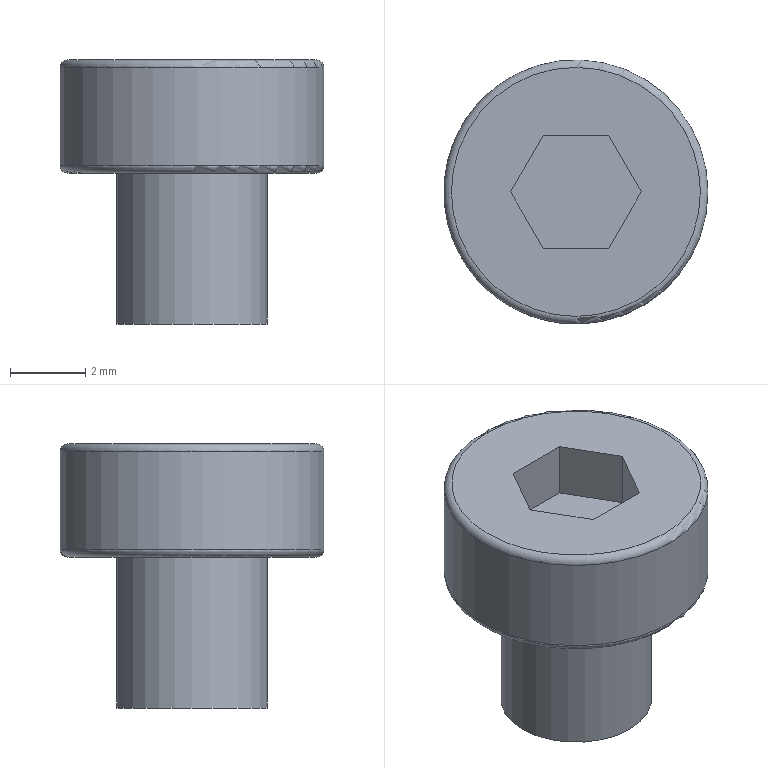Part | STEP file | Tube feed_id802_x_t | 1 solid | 14 faces | box 7 x 7 x 7 mm | volume 153.655 mm3 | plane 10 | cylinder 2 | torus 2 | commonest cylinder face diameters 4 x1 7 x1
STEP:
#1=CARTESIAN_POINT('',(0.,0.,0.));
#2=DIRECTION('',(0.,0.,1.));
#3=DIRECTION('',(1.,0.,0.));
#4=AXIS2_PLACEMENT_3D('',#1,#2,#3);
#5=CARTESIAN_POINT('',(457.,3.036,-9.8));
#6=VERTEX_POINT('',#5);
#7=CARTESIAN_POINT('',(453.5,3.036,-9.8));
#8=DIRECTION('',(0.,0.,1.));
#9=DIRECTION('',(1.,0.,0.));
#10=AXIS2_PLACEMENT_3D('',#7,#8,#9);
#11=CIRCLE('',#10,3.5);
#12=CARTESIAN_POINT('',(453.5,3.036,-10.));
#13=DIRECTION('',(0.,0.,1.));
#14=DIRECTION('',(1.,0.,0.));
#15=AXIS2_PLACEMENT_3D('',#12,#13,#14);
#16=CYLINDRICAL_SURFACE('',#15,3.5);
#17=CARTESIAN_POINT('',(0.,0.2));
#18=DIRECTION('',(1.,0.));
#19=VECTOR('',#18,1.);
#20=LINE('',#17,#19);
#21=(GEOMETRIC_REPRESENTATION_CONTEXT(2)PARAMETRIC_REPRESENTATION_CONTEXT()REPRESENTATION_CONTEXT('',''));
#22=DEFINITIONAL_REPRESENTATION('',(#20),#21);
#23=PCURVE('',#16,#22);
#24=CARTESIAN_POINT('',(453.5,3.036,-9.8));
#25=DIRECTION('',(0.,0.,1.));
#26=DIRECTION('',(1.,0.,0.));
#27=AXIS2_PLACEMENT_3D('',#24,#25,#26);
#28=TOROIDAL_SURFACE('',#27,3.3,0.2);
#29=CARTESIAN_POINT('',(0.,6.283));
#30=DIRECTION('',(1.,0.));
#31=VECTOR('',#30,1.);
#32=LINE('',#29,#31);
#33=(GEOMETRIC_REPRESENTATION_CONTEXT(2)PARAMETRIC_REPRESENTATION_CONTEXT()REPRESENTATION_CONTEXT('',''));
#34=DEFINITIONAL_REPRESENTATION('',(#32),#33);
#35=PCURVE('',#28,#34);
#36=SURFACE_CURVE('',#11,(#23,#35),.PCURVE_S1.);
#37=EDGE_CURVE('',#6,#6,#36,.T.);
#38=ORIENTED_EDGE('',*,*,#37,.T.);
#39=CARTESIAN_POINT('',(457.,3.036,-7.2));
#40=VERTEX_POINT('',#39);
#41=CARTESIAN_POINT('',(457.,3.036,-9.8));
#42=CARTESIAN_POINT('',(457.,3.036,-7.2));
#43=B_SPLINE_CURVE_WITH_KNOTS('',1,(#41,#42),.UNSPECIFIED.,.F.,.F.,(2,2),(0.2,2.8),.PIECEWISE_BEZIER_KNOTS.);
#44=CARTESIAN_POINT('',(6.283,0.));
#45=DIRECTION('',(0.,1.));
#46=VECTOR('',#45,1.);
#47=LINE('',#44,#46);
#48=(GEOMETRIC_REPRESENTATION_CONTEXT(2)PARAMETRIC_REPRESENTATION_CONTEXT()REPRESENTATION_CONTEXT('',''));
#49=DEFINITIONAL_REPRESENTATION('',(#47),#48);
#50=PCURVE('',#16,#49);
#51=CARTESIAN_POINT('',(0.,0.));
#52=DIRECTION('',(0.,1.));
#53=VECTOR('',#52,1.);
#54=LINE('',#51,#53);
#55=(GEOMETRIC_REPRESENTATION_CONTEXT(2)PARAMETRIC_REPRESENTATION_CONTEXT()REPRESENTATION_CONTEXT('',''));
#56=DEFINITIONAL_REPRESENTATION('',(#54),#55);
#57=PCURVE('',#16,#56);
#58=SEAM_CURVE('',#43,(#50,#57),.PCURVE_S1.);
#59=EDGE_CURVE('',#6,#40,#58,.T.);
#60=ORIENTED_EDGE('',*,*,#59,.T.);
#61=CARTESIAN_POINT('',(453.5,3.036,-7.2));
#62=DIRECTION('',(0.,0.,-1.));
#63=DIRECTION('',(1.,0.,0.));
#64=AXIS2_PLACEMENT_3D('',#61,#62,#63);
#65=CIRCLE('',#64,3.5);
#66=CARTESIAN_POINT('',(6.283,2.8));
#67=DIRECTION('',(-1.,0.));
#68=VECTOR('',#67,1.);
#69=LINE('',#66,#68);
#70=(GEOMETRIC_REPRESENTATION_CONTEXT(2)PARAMETRIC_REPRESENTATION_CONTEXT()REPRESENTATION_CONTEXT('',''));
#71=DEFINITIONAL_REPRESENTATION('',(#69),#70);
#72=PCURVE('',#16,#71);
#73=CARTESIAN_POINT('',(453.5,3.036,-7.2));
#74=DIRECTION('',(0.,0.,1.));
#75=DIRECTION('',(1.,0.,0.));
#76=AXIS2_PLACEMENT_3D('',#73,#74,#75);
#77=TOROIDAL_SURFACE('',#76,3.3,0.2);
#78=CARTESIAN_POINT('',(6.283,6.283));
#79=DIRECTION('',(-1.,0.));
#80=VECTOR('',#79,1.);
#81=LINE('',#78,#80);
#82=(GEOMETRIC_REPRESENTATION_CONTEXT(2)PARAMETRIC_REPRESENTATION_CONTEXT()REPRESENTATION_CONTEXT('',''));
#83=DEFINITIONAL_REPRESENTATION('',(#81),#82);
#84=PCURVE('',#77,#83);
#85=SURFACE_CURVE('',#65,(#72,#84),.PCURVE_S1.);
#86=EDGE_CURVE('',#40,#40,#85,.T.);
#87=ORIENTED_EDGE('',*,*,#86,.T.);
#88=ORIENTED_EDGE('',*,*,#59,.F.);
#89=EDGE_LOOP('',(#38,#60,#87,#88));
#90=FACE_BOUND('',#89,.T.);
#91=ADVANCED_FACE('',(#90),#16,.T.);
#92=CARTESIAN_POINT('',(451.5,3.036,-10.));
#93=VERTEX_POINT('',#92);
#94=CARTESIAN_POINT('',(453.5,3.036,-10.));
#95=DIRECTION('',(0.,0.,-1.));
#96=DIRECTION('',(-1.,0.,0.));
#97=AXIS2_PLACEMENT_3D('',#94,#95,#96);
#98=CIRCLE('',#97,2.);
#99=CARTESIAN_POINT('',(453.5,3.036,-10.));
#100=DIRECTION('',(0.,0.,1.));
#101=DIRECTION('',(1.,0.,0.));
#102=AXIS2_PLACEMENT_3D('',#99,#100,#101);
#103=PLANE('',#102);
#104=CARTESIAN_POINT('',(-2.,0.));
#105=CARTESIAN_POINT('',(-2.,3.464));
#106=CARTESIAN_POINT('',(1.,1.732));
#107=CARTESIAN_POINT('',(4.,0.));
#108=CARTESIAN_POINT('',(1.,-1.732));
#109=CARTESIAN_POINT('',(-2.,-3.464));
#110=CARTESIAN_POINT('',(-2.,0.));
#111=(BOUNDED_CURVE()B_SPLINE_CURVE(2,(#104,#105,#106,#107,#108,#109,#110),.UNSPECIFIED.,.T.,.F.)B_SPLINE_CURVE_WITH_KNOTS((1,2,2,2,2,1),(-2.094,0.,2.094,4.189,6.283,8.378),.UNSPECIFIED.)CURVE()GEOMETRIC_REPRESENTATION_ITEM()RATIONAL_B_SPLINE_CURVE((1.,0.5,1.,0.5,1.,0.5,1.))REPRESENTATION_ITEM(''));
#112=(GEOMETRIC_REPRESENTATION_CONTEXT(2)PARAMETRIC_REPRESENTATION_CONTEXT()REPRESENTATION_CONTEXT('',''));
#113=DEFINITIONAL_REPRESENTATION('',(#111),#112);
#114=PCURVE('',#103,#113);
#115=CARTESIAN_POINT('',(453.5,3.036,-14.));
#116=DIRECTION('',(0.,0.,1.));
#117=DIRECTION('',(1.,0.,0.));
#118=AXIS2_PLACEMENT_3D('',#115,#116,#117);
#119=CYLINDRICAL_SURFACE('',#118,2.);
#120=CARTESIAN_POINT('',(9.425,4.));
#121=DIRECTION('',(-1.,0.));
#122=VECTOR('',#121,1.);
#123=LINE('',#120,#122);
#124=(GEOMETRIC_REPRESENTATION_CONTEXT(2)PARAMETRIC_REPRESENTATION_CONTEXT()REPRESENTATION_CONTEXT('',''));
#125=DEFINITIONAL_REPRESENTATION('',(#123),#124);
#126=PCURVE('',#119,#125);
#127=SURFACE_CURVE('',#98,(#114,#126),.PCURVE_S1.);
#128=EDGE_CURVE('',#93,#93,#127,.T.);
#129=ORIENTED_EDGE('',*,*,#128,.F.);
#130=EDGE_LOOP('',(#129));
#131=FACE_BOUND('',#130,.T.);
#132=CARTESIAN_POINT('',(456.8,3.036,-10.));
#133=VERTEX_POINT('',#132);
#134=CARTESIAN_POINT('',(453.5,3.036,-10.));
#135=DIRECTION('',(0.,0.,-1.));
#136=DIRECTION('',(1.,0.,0.));
#137=AXIS2_PLACEMENT_3D('',#134,#135,#136);
#138=CIRCLE('',#137,3.3);
#139=CARTESIAN_POINT('',(3.3,0.));
#140=CARTESIAN_POINT('',(3.3,-5.716));
#141=CARTESIAN_POINT('',(-1.65,-2.858));
#142=CARTESIAN_POINT('',(-6.6,0.));
#143=CARTESIAN_POINT('',(-1.65,2.858));
#144=CARTESIAN_POINT('',(3.3,5.716));
#145=CARTESIAN_POINT('',(3.3,0.));
#146=(BOUNDED_CURVE()B_SPLINE_CURVE(2,(#139,#140,#141,#142,#143,#144,#145),.UNSPECIFIED.,.T.,.F.)B_SPLINE_CURVE_WITH_KNOTS((1,2,2,2,2,1),(-2.094,0.,2.094,4.189,6.283,8.378),.UNSPECIFIED.)CURVE()GEOMETRIC_REPRESENTATION_ITEM()RATIONAL_B_SPLINE_CURVE((1.,0.5,1.,0.5,1.,0.5,1.))REPRESENTATION_ITEM(''));
#147=(GEOMETRIC_REPRESENTATION_CONTEXT(2)PARAMETRIC_REPRESENTATION_CONTEXT()REPRESENTATION_CONTEXT('',''));
#148=DEFINITIONAL_REPRESENTATION('',(#146),#147);
#149=PCURVE('',#103,#148);
#150=CARTESIAN_POINT('',(6.283,4.712));
#151=DIRECTION('',(-1.,0.));
#152=VECTOR('',#151,1.);
#153=LINE('',#150,#152);
#154=(GEOMETRIC_REPRESENTATION_CONTEXT(2)PARAMETRIC_REPRESENTATION_CONTEXT()REPRESENTATION_CONTEXT('',''));
#155=DEFINITIONAL_REPRESENTATION('',(#153),#154);
#156=PCURVE('',#28,#155);
#157=SURFACE_CURVE('',#138,(#149,#156),.PCURVE_S1.);
#158=EDGE_CURVE('',#133,#133,#157,.T.);
#159=ORIENTED_EDGE('',*,*,#158,.T.);
#160=EDGE_LOOP('',(#159));
#161=FACE_BOUND('',#160,.T.);
#162=ADVANCED_FACE('',(#131,#161),#103,.F.);
#163=CARTESIAN_POINT('',(451.768,3.036,-7.));
#164=VERTEX_POINT('',#163);
#165=CARTESIAN_POINT('',(452.634,1.536,-7.));
#166=VERTEX_POINT('',#165);
#167=CARTESIAN_POINT('',(451.768,3.036,-7.));
#168=DIRECTION('',(0.5,-0.866,0.));
#169=VECTOR('',#168,1.);
#170=LINE('',#167,#169);
#171=CARTESIAN_POINT('',(453.5,3.036,-7.));
#172=DIRECTION('',(0.,0.,1.));
#173=DIRECTION('',(1.,0.,0.));
#174=AXIS2_PLACEMENT_3D('',#171,#172,#173);
#175=PLANE('',#174);
#176=CARTESIAN_POINT('',(-1.732,0.));
#177=DIRECTION('',(0.5,-0.866));
#178=VECTOR('',#177,1.);
#179=LINE('',#176,#178);
#180=(GEOMETRIC_REPRESENTATION_CONTEXT(2)PARAMETRIC_REPRESENTATION_CONTEXT()REPRESENTATION_CONTEXT('',''));
#181=DEFINITIONAL_REPRESENTATION('',(#179),#180);
#182=PCURVE('',#175,#181);
#183=CARTESIAN_POINT('',(451.768,3.036,-8.5));
#184=DIRECTION('',(-0.866,-0.5,0.));
#185=DIRECTION('',(0.5,-0.866,0.));
#186=AXIS2_PLACEMENT_3D('',#183,#184,#185);
#187=PLANE('',#186);
#188=CARTESIAN_POINT('',(0.,1.5));
#189=DIRECTION('',(1.,0.));
#190=VECTOR('',#189,1.);
#191=LINE('',#188,#190);
#192=(GEOMETRIC_REPRESENTATION_CONTEXT(2)PARAMETRIC_REPRESENTATION_CONTEXT()REPRESENTATION_CONTEXT('',''));
#193=DEFINITIONAL_REPRESENTATION('',(#191),#192);
#194=PCURVE('',#187,#193);
#195=SURFACE_CURVE('',#170,(#182,#194),.PCURVE_S1.);
#196=EDGE_CURVE('',#164,#166,#195,.T.);
#197=ORIENTED_EDGE('',*,*,#196,.F.);
#198=CARTESIAN_POINT('',(452.634,4.536,-7.));
#199=VERTEX_POINT('',#198);
#200=CARTESIAN_POINT('',(452.634,4.536,-7.));
#201=DIRECTION('',(-0.5,-0.866,0.));
#202=VECTOR('',#201,1.);
#203=LINE('',#200,#202);
#204=CARTESIAN_POINT('',(-0.866,1.5));
#205=DIRECTION('',(-0.5,-0.866));
#206=VECTOR('',#205,1.);
#207=LINE('',#204,#206);
#208=(GEOMETRIC_REPRESENTATION_CONTEXT(2)PARAMETRIC_REPRESENTATION_CONTEXT()REPRESENTATION_CONTEXT('',''));
#209=DEFINITIONAL_REPRESENTATION('',(#207),#208);
#210=PCURVE('',#175,#209);
#211=CARTESIAN_POINT('',(452.634,4.536,-8.5));
#212=DIRECTION('',(-0.866,0.5,0.));
#213=DIRECTION('',(-0.5,-0.866,0.));
#214=AXIS2_PLACEMENT_3D('',#211,#212,#213);
#215=PLANE('',#214);
#216=CARTESIAN_POINT('',(0.,1.5));
#217=DIRECTION('',(1.,0.));
#218=VECTOR('',#217,1.);
#219=LINE('',#216,#218);
#220=(GEOMETRIC_REPRESENTATION_CONTEXT(2)PARAMETRIC_REPRESENTATION_CONTEXT()REPRESENTATION_CONTEXT('',''));
#221=DEFINITIONAL_REPRESENTATION('',(#219),#220);
#222=PCURVE('',#215,#221);
#223=SURFACE_CURVE('',#203,(#210,#222),.PCURVE_S1.);
#224=EDGE_CURVE('',#199,#164,#223,.T.);
#225=ORIENTED_EDGE('',*,*,#224,.F.);
#226=CARTESIAN_POINT('',(454.366,4.536,-7.));
#227=VERTEX_POINT('',#226);
#228=CARTESIAN_POINT('',(454.366,4.536,-7.));
#229=DIRECTION('',(-1.,0.,0.));
#230=VECTOR('',#229,1.);
#231=LINE('',#228,#230);
#232=CARTESIAN_POINT('',(0.866,1.5));
#233=DIRECTION('',(-1.,0.));
#234=VECTOR('',#233,1.);
#235=LINE('',#232,#234);
#236=(GEOMETRIC_REPRESENTATION_CONTEXT(2)PARAMETRIC_REPRESENTATION_CONTEXT()REPRESENTATION_CONTEXT('',''));
#237=DEFINITIONAL_REPRESENTATION('',(#235),#236);
#238=PCURVE('',#175,#237);
#239=CARTESIAN_POINT('',(454.366,4.536,-8.5));
#240=DIRECTION('',(0.,1.,0.));
#241=DIRECTION('',(0.,0.,1.));
#242=AXIS2_PLACEMENT_3D('',#239,#240,#241);
#243=PLANE('',#242);
#244=CARTESIAN_POINT('',(1.5,0.));
#245=DIRECTION('',(0.,-1.));
#246=VECTOR('',#245,1.);
#247=LINE('',#244,#246);
#248=(GEOMETRIC_REPRESENTATION_CONTEXT(2)PARAMETRIC_REPRESENTATION_CONTEXT()REPRESENTATION_CONTEXT('',''));
#249=DEFINITIONAL_REPRESENTATION('',(#247),#248);
#250=PCURVE('',#243,#249);
#251=SURFACE_CURVE('',#231,(#238,#250),.PCURVE_S1.);
#252=EDGE_CURVE('',#227,#199,#251,.T.);
#253=ORIENTED_EDGE('',*,*,#252,.F.);
#254=CARTESIAN_POINT('',(455.232,3.036,-7.));
#255=VERTEX_POINT('',#254);
#256=CARTESIAN_POINT('',(455.232,3.036,-7.));
#257=DIRECTION('',(-0.5,0.866,0.));
#258=VECTOR('',#257,1.);
#259=LINE('',#256,#258);
#260=CARTESIAN_POINT('',(1.732,0.));
#261=DIRECTION('',(-0.5,0.866));
#262=VECTOR('',#261,1.);
#263=LINE('',#260,#262);
#264=(GEOMETRIC_REPRESENTATION_CONTEXT(2)PARAMETRIC_REPRESENTATION_CONTEXT()REPRESENTATION_CONTEXT('',''));
#265=DEFINITIONAL_REPRESENTATION('',(#263),#264);
#266=PCURVE('',#175,#265);
#267=CARTESIAN_POINT('',(455.232,3.036,-8.5));
#268=DIRECTION('',(0.866,0.5,0.));
#269=DIRECTION('',(-0.5,0.866,0.));
#270=AXIS2_PLACEMENT_3D('',#267,#268,#269);
#271=PLANE('',#270);
#272=CARTESIAN_POINT('',(0.,1.5));
#273=DIRECTION('',(1.,0.));
#274=VECTOR('',#273,1.);
#275=LINE('',#272,#274);
#276=(GEOMETRIC_REPRESENTATION_CONTEXT(2)PARAMETRIC_REPRESENTATION_CONTEXT()REPRESENTATION_CONTEXT('',''));
#277=DEFINITIONAL_REPRESENTATION('',(#275),#276);
#278=PCURVE('',#271,#277);
#279=SURFACE_CURVE('',#259,(#266,#278),.PCURVE_S1.);
#280=EDGE_CURVE('',#255,#227,#279,.T.);
#281=ORIENTED_EDGE('',*,*,#280,.F.);
#282=CARTESIAN_POINT('',(454.366,1.536,-7.));
#283=VERTEX_POINT('',#282);
#284=CARTESIAN_POINT('',(454.366,1.536,-7.));
#285=DIRECTION('',(0.5,0.866,0.));
#286=VECTOR('',#285,1.);
#287=LINE('',#284,#286);
#288=CARTESIAN_POINT('',(0.866,-1.5));
#289=DIRECTION('',(0.5,0.866));
#290=VECTOR('',#289,1.);
#291=LINE('',#288,#290);
#292=(GEOMETRIC_REPRESENTATION_CONTEXT(2)PARAMETRIC_REPRESENTATION_CONTEXT()REPRESENTATION_CONTEXT('',''));
#293=DEFINITIONAL_REPRESENTATION('',(#291),#292);
#294=PCURVE('',#175,#293);
#295=CARTESIAN_POINT('',(454.366,1.536,-8.5));
#296=DIRECTION('',(0.866,-0.5,0.));
#297=DIRECTION('',(0.5,0.866,0.));
#298=AXIS2_PLACEMENT_3D('',#295,#296,#297);
#299=PLANE('',#298);
#300=CARTESIAN_POINT('',(0.,1.5));
#301=DIRECTION('',(1.,0.));
#302=VECTOR('',#301,1.);
#303=LINE('',#300,#302);
#304=(GEOMETRIC_REPRESENTATION_CONTEXT(2)PARAMETRIC_REPRESENTATION_CONTEXT()REPRESENTATION_CONTEXT('',''));
#305=DEFINITIONAL_REPRESENTATION('',(#303),#304);
#306=PCURVE('',#299,#305);
#307=SURFACE_CURVE('',#287,(#294,#306),.PCURVE_S1.);
#308=EDGE_CURVE('',#283,#255,#307,.T.);
#309=ORIENTED_EDGE('',*,*,#308,.F.);
#310=CARTESIAN_POINT('',(452.634,1.536,-7.));
#311=DIRECTION('',(1.,0.,0.));
#312=VECTOR('',#311,1.);
#313=LINE('',#310,#312);
#314=CARTESIAN_POINT('',(-0.866,-1.5));
#315=DIRECTION('',(1.,0.));
#316=VECTOR('',#315,1.);
#317=LINE('',#314,#316);
#318=(GEOMETRIC_REPRESENTATION_CONTEXT(2)PARAMETRIC_REPRESENTATION_CONTEXT()REPRESENTATION_CONTEXT('',''));
#319=DEFINITIONAL_REPRESENTATION('',(#317),#318);
#320=PCURVE('',#175,#319);
#321=CARTESIAN_POINT('',(452.634,1.536,-8.5));
#322=DIRECTION('',(0.,-1.,0.));
#323=DIRECTION('',(0.,0.,-1.));
#324=AXIS2_PLACEMENT_3D('',#321,#322,#323);
#325=PLANE('',#324);
#326=CARTESIAN_POINT('',(-1.5,0.));
#327=DIRECTION('',(0.,1.));
#328=VECTOR('',#327,1.);
#329=LINE('',#326,#328);
#330=(GEOMETRIC_REPRESENTATION_CONTEXT(2)PARAMETRIC_REPRESENTATION_CONTEXT()REPRESENTATION_CONTEXT('',''));
#331=DEFINITIONAL_REPRESENTATION('',(#329),#330);
#332=PCURVE('',#325,#331);
#333=SURFACE_CURVE('',#313,(#320,#332),.PCURVE_S1.);
#334=EDGE_CURVE('',#166,#283,#333,.T.);
#335=ORIENTED_EDGE('',*,*,#334,.F.);
#336=EDGE_LOOP('',(#197,#225,#253,#281,#309,#335));
#337=FACE_BOUND('',#336,.T.);
#338=CARTESIAN_POINT('',(456.8,3.036,-7.));
#339=VERTEX_POINT('',#338);
#340=CARTESIAN_POINT('',(453.5,3.036,-7.));
#341=DIRECTION('',(0.,0.,1.));
#342=DIRECTION('',(1.,0.,0.));
#343=AXIS2_PLACEMENT_3D('',#340,#341,#342);
#344=CIRCLE('',#343,3.3);
#345=CARTESIAN_POINT('',(0.,0.));
#346=DIRECTION('',(1.,0.));
#347=AXIS2_PLACEMENT_2D('',#345,#346);
#348=CIRCLE('',#347,3.3);
#349=(GEOMETRIC_REPRESENTATION_CONTEXT(2)PARAMETRIC_REPRESENTATION_CONTEXT()REPRESENTATION_CONTEXT('',''));
#350=DEFINITIONAL_REPRESENTATION('',(#348),#349);
#351=PCURVE('',#175,#350);
#352=CARTESIAN_POINT('',(0.,7.854));
#353=DIRECTION('',(1.,0.));
#354=VECTOR('',#353,1.);
#355=LINE('',#352,#354);
#356=(GEOMETRIC_REPRESENTATION_CONTEXT(2)PARAMETRIC_REPRESENTATION_CONTEXT()REPRESENTATION_CONTEXT('',''));
#357=DEFINITIONAL_REPRESENTATION('',(#355),#356);
#358=PCURVE('',#77,#357);
#359=SURFACE_CURVE('',#344,(#351,#358),.PCURVE_S1.);
#360=EDGE_CURVE('',#339,#339,#359,.T.);
#361=ORIENTED_EDGE('',*,*,#360,.T.);
#362=EDGE_LOOP('',(#361));
#363=FACE_BOUND('',#362,.T.);
#364=ADVANCED_FACE('',(#337,#363),#175,.T.);
#365=ORIENTED_EDGE('',*,*,#158,.F.);
#366=CARTESIAN_POINT('',(456.8,3.036,-10.));
#367=CARTESIAN_POINT('',(456.853,3.036,-10.));
#368=CARTESIAN_POINT('',(456.906,3.036,-9.983));
#369=CARTESIAN_POINT('',(456.95,3.036,-9.95));
#370=CARTESIAN_POINT('',(456.983,3.036,-9.906));
#371=CARTESIAN_POINT('',(457.,3.036,-9.853));
#372=CARTESIAN_POINT('',(457.,3.036,-9.8));
#373=(BOUNDED_CURVE()B_SPLINE_CURVE(6,(#366,#367,#368,#369,#370,#371,#372),.UNSPECIFIED.,.F.,.F.)B_SPLINE_CURVE_WITH_KNOTS((7,7),(4.712,6.283),.PIECEWISE_BEZIER_KNOTS.)CURVE()GEOMETRIC_REPRESENTATION_ITEM()RATIONAL_B_SPLINE_CURVE((1.031,1.01,0.9979,0.994,0.9979,1.01,1.031))REPRESENTATION_ITEM(''));
#374=CARTESIAN_POINT('',(6.283,0.));
#375=DIRECTION('',(0.,1.));
#376=VECTOR('',#375,1.);
#377=LINE('',#374,#376);
#378=(GEOMETRIC_REPRESENTATION_CONTEXT(2)PARAMETRIC_REPRESENTATION_CONTEXT()REPRESENTATION_CONTEXT('',''));
#379=DEFINITIONAL_REPRESENTATION('',(#377),#378);
#380=PCURVE('',#28,#379);
#381=CARTESIAN_POINT('',(0.,0.));
#382=DIRECTION('',(0.,1.));
#383=VECTOR('',#382,1.);
#384=LINE('',#381,#383);
#385=(GEOMETRIC_REPRESENTATION_CONTEXT(2)PARAMETRIC_REPRESENTATION_CONTEXT()REPRESENTATION_CONTEXT('',''));
#386=DEFINITIONAL_REPRESENTATION('',(#384),#385);
#387=PCURVE('',#28,#386);
#388=SEAM_CURVE('',#373,(#380,#387),.PCURVE_S1.);
#389=EDGE_CURVE('',#133,#6,#388,.T.);
#390=ORIENTED_EDGE('',*,*,#389,.T.);
#391=ORIENTED_EDGE('',*,*,#37,.F.);
#392=ORIENTED_EDGE('',*,*,#389,.F.);
#393=EDGE_LOOP('',(#365,#390,#391,#392));
#394=FACE_BOUND('',#393,.T.);
#395=ADVANCED_FACE('',(#394),#28,.T.);
#396=ORIENTED_EDGE('',*,*,#86,.F.);
#397=CARTESIAN_POINT('',(457.,3.036,-7.2));
#398=CARTESIAN_POINT('',(457.,3.036,-7.147));
#399=CARTESIAN_POINT('',(456.983,3.036,-7.094));
#400=CARTESIAN_POINT('',(456.95,3.036,-7.05));
#401=CARTESIAN_POINT('',(456.906,3.036,-7.017));
#402=CARTESIAN_POINT('',(456.853,3.036,-7.));
#403=CARTESIAN_POINT('',(456.8,3.036,-7.));
#404=(BOUNDED_CURVE()B_SPLINE_CURVE(6,(#397,#398,#399,#400,#401,#402,#403),.UNSPECIFIED.,.F.,.F.)B_SPLINE_CURVE_WITH_KNOTS((7,7),(0.,1.571),.PIECEWISE_BEZIER_KNOTS.)CURVE()GEOMETRIC_REPRESENTATION_ITEM()RATIONAL_B_SPLINE_CURVE((1.031,1.01,0.9979,0.994,0.9979,1.01,1.031))REPRESENTATION_ITEM(''));
#405=CARTESIAN_POINT('',(6.283,6.283));
#406=DIRECTION('',(0.,1.));
#407=VECTOR('',#406,1.);
#408=LINE('',#405,#407);
#409=(GEOMETRIC_REPRESENTATION_CONTEXT(2)PARAMETRIC_REPRESENTATION_CONTEXT()REPRESENTATION_CONTEXT('',''));
#410=DEFINITIONAL_REPRESENTATION('',(#408),#409);
#411=PCURVE('',#77,#410);
#412=CARTESIAN_POINT('',(0.,6.283));
#413=DIRECTION('',(0.,1.));
#414=VECTOR('',#413,1.);
#415=LINE('',#412,#414);
#416=(GEOMETRIC_REPRESENTATION_CONTEXT(2)PARAMETRIC_REPRESENTATION_CONTEXT()REPRESENTATION_CONTEXT('',''));
#417=DEFINITIONAL_REPRESENTATION('',(#415),#416);
#418=PCURVE('',#77,#417);
#419=SEAM_CURVE('',#404,(#411,#418),.PCURVE_S1.);
#420=EDGE_CURVE('',#40,#339,#419,.T.);
#421=ORIENTED_EDGE('',*,*,#420,.T.);
#422=ORIENTED_EDGE('',*,*,#360,.F.);
#423=ORIENTED_EDGE('',*,*,#420,.F.);
#424=EDGE_LOOP('',(#396,#421,#422,#423));
#425=FACE_BOUND('',#424,.T.);
#426=ADVANCED_FACE('',(#425),#77,.T.);
#427=ORIENTED_EDGE('',*,*,#196,.T.);
#428=CARTESIAN_POINT('',(452.634,1.536,-8.5));
#429=VERTEX_POINT('',#428);
#430=CARTESIAN_POINT('',(452.634,1.536,-8.5));
#431=DIRECTION('',(0.,0.,-1.));
#432=VECTOR('',#431,1.);
#433=LINE('',#430,#432);
#434=CARTESIAN_POINT('',(1.732,0.));
#435=DIRECTION('',(0.,-1.));
#436=VECTOR('',#435,1.);
#437=LINE('',#434,#436);
#438=(GEOMETRIC_REPRESENTATION_CONTEXT(2)PARAMETRIC_REPRESENTATION_CONTEXT()REPRESENTATION_CONTEXT('',''));
#439=DEFINITIONAL_REPRESENTATION('',(#437),#438);
#440=PCURVE('',#187,#439);
#441=CARTESIAN_POINT('',(0.,0.));
#442=DIRECTION('',(1.,0.));
#443=VECTOR('',#442,1.);
#444=LINE('',#441,#443);
#445=(GEOMETRIC_REPRESENTATION_CONTEXT(2)PARAMETRIC_REPRESENTATION_CONTEXT()REPRESENTATION_CONTEXT('',''));
#446=DEFINITIONAL_REPRESENTATION('',(#444),#445);
#447=PCURVE('',#325,#446);
#448=SURFACE_CURVE('',#433,(#440,#447),.PCURVE_S1.);
#449=EDGE_CURVE('',#166,#429,#448,.T.);
#450=ORIENTED_EDGE('',*,*,#449,.T.);
#451=CARTESIAN_POINT('',(451.768,3.036,-8.5));
#452=VERTEX_POINT('',#451);
#453=CARTESIAN_POINT('',(451.768,3.036,-8.5));
#454=DIRECTION('',(-0.5,0.866,0.));
#455=VECTOR('',#454,1.);
#456=LINE('',#453,#455);
#457=CARTESIAN_POINT('',(0.,0.));
#458=DIRECTION('',(-1.,0.));
#459=VECTOR('',#458,1.);
#460=LINE('',#457,#459);
#461=(GEOMETRIC_REPRESENTATION_CONTEXT(2)PARAMETRIC_REPRESENTATION_CONTEXT()REPRESENTATION_CONTEXT('',''));
#462=DEFINITIONAL_REPRESENTATION('',(#460),#461);
#463=PCURVE('',#187,#462);
#464=CARTESIAN_POINT('',(0.,0.,-8.5));
#465=DIRECTION('',(0.,0.,1.));
#466=DIRECTION('',(1.,0.,0.));
#467=AXIS2_PLACEMENT_3D('',#464,#465,#466);
#468=PLANE('',#467);
#469=CARTESIAN_POINT('',(451.768,3.036));
#470=DIRECTION('',(-0.5,0.866));
#471=VECTOR('',#470,1.);
#472=LINE('',#469,#471);
#473=(GEOMETRIC_REPRESENTATION_CONTEXT(2)PARAMETRIC_REPRESENTATION_CONTEXT()REPRESENTATION_CONTEXT('',''));
#474=DEFINITIONAL_REPRESENTATION('',(#472),#473);
#475=PCURVE('',#468,#474);
#476=SURFACE_CURVE('',#456,(#463,#475),.PCURVE_S1.);
#477=EDGE_CURVE('',#429,#452,#476,.T.);
#478=ORIENTED_EDGE('',*,*,#477,.T.);
#479=CARTESIAN_POINT('',(451.768,3.036,-8.5));
#480=DIRECTION('',(0.,0.,-1.));
#481=VECTOR('',#480,1.);
#482=LINE('',#479,#481);
#483=CARTESIAN_POINT('',(0.,0.));
#484=DIRECTION('',(0.,-1.));
#485=VECTOR('',#484,1.);
#486=LINE('',#483,#485);
#487=(GEOMETRIC_REPRESENTATION_CONTEXT(2)PARAMETRIC_REPRESENTATION_CONTEXT()REPRESENTATION_CONTEXT('',''));
#488=DEFINITIONAL_REPRESENTATION('',(#486),#487);
#489=PCURVE('',#187,#488);
#490=CARTESIAN_POINT('',(1.732,0.));
#491=DIRECTION('',(0.,-1.));
#492=VECTOR('',#491,1.);
#493=LINE('',#490,#492);
#494=(GEOMETRIC_REPRESENTATION_CONTEXT(2)PARAMETRIC_REPRESENTATION_CONTEXT()REPRESENTATION_CONTEXT('',''));
#495=DEFINITIONAL_REPRESENTATION('',(#493),#494);
#496=PCURVE('',#215,#495);
#497=SURFACE_CURVE('',#482,(#489,#496),.PCURVE_S1.);
#498=EDGE_CURVE('',#164,#452,#497,.T.);
#499=ORIENTED_EDGE('',*,*,#498,.F.);
#500=EDGE_LOOP('',(#427,#450,#478,#499));
#501=FACE_BOUND('',#500,.T.);
#502=ADVANCED_FACE('',(#501),#187,.F.);
#503=ORIENTED_EDGE('',*,*,#334,.T.);
#504=CARTESIAN_POINT('',(454.366,1.536,-8.5));
#505=VERTEX_POINT('',#504);
#506=CARTESIAN_POINT('',(454.366,1.536,-8.5));
#507=DIRECTION('',(0.,0.,-1.));
#508=VECTOR('',#507,1.);
#509=LINE('',#506,#508);
#510=CARTESIAN_POINT('',(0.,1.732));
#511=DIRECTION('',(1.,0.));
#512=VECTOR('',#511,1.);
#513=LINE('',#510,#512);
#514=(GEOMETRIC_REPRESENTATION_CONTEXT(2)PARAMETRIC_REPRESENTATION_CONTEXT()REPRESENTATION_CONTEXT('',''));
#515=DEFINITIONAL_REPRESENTATION('',(#513),#514);
#516=PCURVE('',#325,#515);
#517=CARTESIAN_POINT('',(0.,0.));
#518=DIRECTION('',(0.,-1.));
#519=VECTOR('',#518,1.);
#520=LINE('',#517,#519);
#521=(GEOMETRIC_REPRESENTATION_CONTEXT(2)PARAMETRIC_REPRESENTATION_CONTEXT()REPRESENTATION_CONTEXT('',''));
#522=DEFINITIONAL_REPRESENTATION('',(#520),#521);
#523=PCURVE('',#299,#522);
#524=SURFACE_CURVE('',#509,(#516,#523),.PCURVE_S1.);
#525=EDGE_CURVE('',#283,#505,#524,.T.);
#526=ORIENTED_EDGE('',*,*,#525,.T.);
#527=CARTESIAN_POINT('',(452.634,1.536,-8.5));
#528=DIRECTION('',(-1.,0.,0.));
#529=VECTOR('',#528,1.);
#530=LINE('',#527,#529);
#531=CARTESIAN_POINT('',(0.,0.));
#532=DIRECTION('',(0.,-1.));
#533=VECTOR('',#532,1.);
#534=LINE('',#531,#533);
#535=(GEOMETRIC_REPRESENTATION_CONTEXT(2)PARAMETRIC_REPRESENTATION_CONTEXT()REPRESENTATION_CONTEXT('',''));
#536=DEFINITIONAL_REPRESENTATION('',(#534),#535);
#537=PCURVE('',#325,#536);
#538=CARTESIAN_POINT('',(452.634,1.536));
#539=DIRECTION('',(-1.,0.));
#540=VECTOR('',#539,1.);
#541=LINE('',#538,#540);
#542=(GEOMETRIC_REPRESENTATION_CONTEXT(2)PARAMETRIC_REPRESENTATION_CONTEXT()REPRESENTATION_CONTEXT('',''));
#543=DEFINITIONAL_REPRESENTATION('',(#541),#542);
#544=PCURVE('',#468,#543);
#545=SURFACE_CURVE('',#530,(#537,#544),.PCURVE_S1.);
#546=EDGE_CURVE('',#505,#429,#545,.T.);
#547=ORIENTED_EDGE('',*,*,#546,.T.);
#548=ORIENTED_EDGE('',*,*,#449,.F.);
#549=EDGE_LOOP('',(#503,#526,#547,#548));
#550=FACE_BOUND('',#549,.T.);
#551=ADVANCED_FACE('',(#550),#325,.F.);
#552=ORIENTED_EDGE('',*,*,#308,.T.);
#553=CARTESIAN_POINT('',(455.232,3.036,-8.5));
#554=VERTEX_POINT('',#553);
#555=CARTESIAN_POINT('',(455.232,3.036,-8.5));
#556=DIRECTION('',(0.,0.,-1.));
#557=VECTOR('',#556,1.);
#558=LINE('',#555,#557);
#559=CARTESIAN_POINT('',(1.732,0.));
#560=DIRECTION('',(0.,-1.));
#561=VECTOR('',#560,1.);
#562=LINE('',#559,#561);
#563=(GEOMETRIC_REPRESENTATION_CONTEXT(2)PARAMETRIC_REPRESENTATION_CONTEXT()REPRESENTATION_CONTEXT('',''));
#564=DEFINITIONAL_REPRESENTATION('',(#562),#563);
#565=PCURVE('',#299,#564);
#566=CARTESIAN_POINT('',(0.,0.));
#567=DIRECTION('',(0.,-1.));
#568=VECTOR('',#567,1.);
#569=LINE('',#566,#568);
#570=(GEOMETRIC_REPRESENTATION_CONTEXT(2)PARAMETRIC_REPRESENTATION_CONTEXT()REPRESENTATION_CONTEXT('',''));
#571=DEFINITIONAL_REPRESENTATION('',(#569),#570);
#572=PCURVE('',#271,#571);
#573=SURFACE_CURVE('',#558,(#565,#572),.PCURVE_S1.);
#574=EDGE_CURVE('',#255,#554,#573,.T.);
#575=ORIENTED_EDGE('',*,*,#574,.T.);
#576=CARTESIAN_POINT('',(454.366,1.536,-8.5));
#577=DIRECTION('',(-0.5,-0.866,0.));
#578=VECTOR('',#577,1.);
#579=LINE('',#576,#578);
#580=CARTESIAN_POINT('',(0.,0.));
#581=DIRECTION('',(-1.,0.));
#582=VECTOR('',#581,1.);
#583=LINE('',#580,#582);
#584=(GEOMETRIC_REPRESENTATION_CONTEXT(2)PARAMETRIC_REPRESENTATION_CONTEXT()REPRESENTATION_CONTEXT('',''));
#585=DEFINITIONAL_REPRESENTATION('',(#583),#584);
#586=PCURVE('',#299,#585);
#587=CARTESIAN_POINT('',(454.366,1.536));
#588=DIRECTION('',(-0.5,-0.866));
#589=VECTOR('',#588,1.);
#590=LINE('',#587,#589);
#591=(GEOMETRIC_REPRESENTATION_CONTEXT(2)PARAMETRIC_REPRESENTATION_CONTEXT()REPRESENTATION_CONTEXT('',''));
#592=DEFINITIONAL_REPRESENTATION('',(#590),#591);
#593=PCURVE('',#468,#592);
#594=SURFACE_CURVE('',#579,(#586,#593),.PCURVE_S1.);
#595=EDGE_CURVE('',#554,#505,#594,.T.);
#596=ORIENTED_EDGE('',*,*,#595,.T.);
#597=ORIENTED_EDGE('',*,*,#525,.F.);
#598=EDGE_LOOP('',(#552,#575,#596,#597));
#599=FACE_BOUND('',#598,.T.);
#600=ADVANCED_FACE('',(#599),#299,.F.);
#601=ORIENTED_EDGE('',*,*,#280,.T.);
#602=CARTESIAN_POINT('',(454.366,4.536,-8.5));
#603=VERTEX_POINT('',#602);
#604=CARTESIAN_POINT('',(454.366,4.536,-8.5));
#605=DIRECTION('',(0.,0.,-1.));
#606=VECTOR('',#605,1.);
#607=LINE('',#604,#606);
#608=CARTESIAN_POINT('',(1.732,0.));
#609=DIRECTION('',(0.,-1.));
#610=VECTOR('',#609,1.);
#611=LINE('',#608,#610);
#612=(GEOMETRIC_REPRESENTATION_CONTEXT(2)PARAMETRIC_REPRESENTATION_CONTEXT()REPRESENTATION_CONTEXT('',''));
#613=DEFINITIONAL_REPRESENTATION('',(#611),#612);
#614=PCURVE('',#271,#613);
#615=CARTESIAN_POINT('',(0.,0.));
#616=DIRECTION('',(-1.,0.));
#617=VECTOR('',#616,1.);
#618=LINE('',#615,#617);
#619=(GEOMETRIC_REPRESENTATION_CONTEXT(2)PARAMETRIC_REPRESENTATION_CONTEXT()REPRESENTATION_CONTEXT('',''));
#620=DEFINITIONAL_REPRESENTATION('',(#618),#619);
#621=PCURVE('',#243,#620);
#622=SURFACE_CURVE('',#607,(#614,#621),.PCURVE_S1.);
#623=EDGE_CURVE('',#227,#603,#622,.T.);
#624=ORIENTED_EDGE('',*,*,#623,.T.);
#625=CARTESIAN_POINT('',(455.232,3.036,-8.5));
#626=DIRECTION('',(0.5,-0.866,0.));
#627=VECTOR('',#626,1.);
#628=LINE('',#625,#627);
#629=CARTESIAN_POINT('',(0.,0.));
#630=DIRECTION('',(-1.,0.));
#631=VECTOR('',#630,1.);
#632=LINE('',#629,#631);
#633=(GEOMETRIC_REPRESENTATION_CONTEXT(2)PARAMETRIC_REPRESENTATION_CONTEXT()REPRESENTATION_CONTEXT('',''));
#634=DEFINITIONAL_REPRESENTATION('',(#632),#633);
#635=PCURVE('',#271,#634);
#636=CARTESIAN_POINT('',(455.232,3.036));
#637=DIRECTION('',(0.5,-0.866));
#638=VECTOR('',#637,1.);
#639=LINE('',#636,#638);
#640=(GEOMETRIC_REPRESENTATION_CONTEXT(2)PARAMETRIC_REPRESENTATION_CONTEXT()REPRESENTATION_CONTEXT('',''));
#641=DEFINITIONAL_REPRESENTATION('',(#639),#640);
#642=PCURVE('',#468,#641);
#643=SURFACE_CURVE('',#628,(#635,#642),.PCURVE_S1.);
#644=EDGE_CURVE('',#603,#554,#643,.T.);
#645=ORIENTED_EDGE('',*,*,#644,.T.);
#646=ORIENTED_EDGE('',*,*,#574,.F.);
#647=EDGE_LOOP('',(#601,#624,#645,#646));
#648=FACE_BOUND('',#647,.T.);
#649=ADVANCED_FACE('',(#648),#271,.F.);
#650=ORIENTED_EDGE('',*,*,#252,.T.);
#651=CARTESIAN_POINT('',(452.634,4.536,-8.5));
#652=VERTEX_POINT('',#651);
#653=CARTESIAN_POINT('',(452.634,4.536,-8.5));
#654=DIRECTION('',(0.,0.,-1.));
#655=VECTOR('',#654,1.);
#656=LINE('',#653,#655);
#657=CARTESIAN_POINT('',(0.,-1.732));
#658=DIRECTION('',(-1.,0.));
#659=VECTOR('',#658,1.);
#660=LINE('',#657,#659);
#661=(GEOMETRIC_REPRESENTATION_CONTEXT(2)PARAMETRIC_REPRESENTATION_CONTEXT()REPRESENTATION_CONTEXT('',''));
#662=DEFINITIONAL_REPRESENTATION('',(#660),#661);
#663=PCURVE('',#243,#662);
#664=CARTESIAN_POINT('',(0.,0.));
#665=DIRECTION('',(0.,-1.));
#666=VECTOR('',#665,1.);
#667=LINE('',#664,#666);
#668=(GEOMETRIC_REPRESENTATION_CONTEXT(2)PARAMETRIC_REPRESENTATION_CONTEXT()REPRESENTATION_CONTEXT('',''));
#669=DEFINITIONAL_REPRESENTATION('',(#667),#668);
#670=PCURVE('',#215,#669);
#671=SURFACE_CURVE('',#656,(#663,#670),.PCURVE_S1.);
#672=EDGE_CURVE('',#199,#652,#671,.T.);
#673=ORIENTED_EDGE('',*,*,#672,.T.);
#674=CARTESIAN_POINT('',(454.366,4.536,-8.5));
#675=DIRECTION('',(1.,0.,0.));
#676=VECTOR('',#675,1.);
#677=LINE('',#674,#676);
#678=CARTESIAN_POINT('',(0.,0.));
#679=DIRECTION('',(0.,1.));
#680=VECTOR('',#679,1.);
#681=LINE('',#678,#680);
#682=(GEOMETRIC_REPRESENTATION_CONTEXT(2)PARAMETRIC_REPRESENTATION_CONTEXT()REPRESENTATION_CONTEXT('',''));
#683=DEFINITIONAL_REPRESENTATION('',(#681),#682);
#684=PCURVE('',#243,#683);
#685=CARTESIAN_POINT('',(454.366,4.536));
#686=DIRECTION('',(1.,0.));
#687=VECTOR('',#686,1.);
#688=LINE('',#685,#687);
#689=(GEOMETRIC_REPRESENTATION_CONTEXT(2)PARAMETRIC_REPRESENTATION_CONTEXT()REPRESENTATION_CONTEXT('',''));
#690=DEFINITIONAL_REPRESENTATION('',(#688),#689);
#691=PCURVE('',#468,#690);
#692=SURFACE_CURVE('',#677,(#684,#691),.PCURVE_S1.);
#693=EDGE_CURVE('',#652,#603,#692,.T.);
#694=ORIENTED_EDGE('',*,*,#693,.T.);
#695=ORIENTED_EDGE('',*,*,#623,.F.);
#696=EDGE_LOOP('',(#650,#673,#694,#695));
#697=FACE_BOUND('',#696,.T.);
#698=ADVANCED_FACE('',(#697),#243,.F.);
#699=ORIENTED_EDGE('',*,*,#224,.T.);
#700=ORIENTED_EDGE('',*,*,#498,.T.);
#701=CARTESIAN_POINT('',(452.634,4.536,-8.5));
#702=DIRECTION('',(0.5,0.866,0.));
#703=VECTOR('',#702,1.);
#704=LINE('',#701,#703);
#705=CARTESIAN_POINT('',(0.,0.));
#706=DIRECTION('',(-1.,0.));
#707=VECTOR('',#706,1.);
#708=LINE('',#705,#707);
#709=(GEOMETRIC_REPRESENTATION_CONTEXT(2)PARAMETRIC_REPRESENTATION_CONTEXT()REPRESENTATION_CONTEXT('',''));
#710=DEFINITIONAL_REPRESENTATION('',(#708),#709);
#711=PCURVE('',#215,#710);
#712=CARTESIAN_POINT('',(452.634,4.536));
#713=DIRECTION('',(0.5,0.866));
#714=VECTOR('',#713,1.);
#715=LINE('',#712,#714);
#716=(GEOMETRIC_REPRESENTATION_CONTEXT(2)PARAMETRIC_REPRESENTATION_CONTEXT()REPRESENTATION_CONTEXT('',''));
#717=DEFINITIONAL_REPRESENTATION('',(#715),#716);
#718=PCURVE('',#468,#717);
#719=SURFACE_CURVE('',#704,(#711,#718),.PCURVE_S1.);
#720=EDGE_CURVE('',#452,#652,#719,.T.);
#721=ORIENTED_EDGE('',*,*,#720,.T.);
#722=ORIENTED_EDGE('',*,*,#672,.F.);
#723=EDGE_LOOP('',(#699,#700,#721,#722));
#724=FACE_BOUND('',#723,.T.);
#725=ADVANCED_FACE('',(#724),#215,.F.);
#726=ORIENTED_EDGE('',*,*,#477,.F.);
#727=ORIENTED_EDGE('',*,*,#546,.F.);
#728=ORIENTED_EDGE('',*,*,#595,.F.);
#729=ORIENTED_EDGE('',*,*,#644,.F.);
#730=ORIENTED_EDGE('',*,*,#693,.F.);
#731=ORIENTED_EDGE('',*,*,#720,.F.);
#732=EDGE_LOOP('',(#726,#727,#728,#729,#730,#731));
#733=FACE_BOUND('',#732,.T.);
#734=ADVANCED_FACE('',(#733),#468,.T.);
#735=CARTESIAN_POINT('',(451.5,3.036,-14.));
#736=VERTEX_POINT('',#735);
#737=CARTESIAN_POINT('',(453.5,3.036,-14.));
#738=DIRECTION('',(0.,0.,-1.));
#739=DIRECTION('',(-1.,0.,0.));
#740=AXIS2_PLACEMENT_3D('',#737,#738,#739);
#741=CIRCLE('',#740,2.);
#742=CARTESIAN_POINT('',(9.425,0.));
#743=DIRECTION('',(-1.,0.));
#744=VECTOR('',#743,1.);
#745=LINE('',#742,#744);
#746=(GEOMETRIC_REPRESENTATION_CONTEXT(2)PARAMETRIC_REPRESENTATION_CONTEXT()REPRESENTATION_CONTEXT('',''));
#747=DEFINITIONAL_REPRESENTATION('',(#745),#746);
#748=PCURVE('',#119,#747);
#749=CARTESIAN_POINT('',(453.5,3.036,-14.));
#750=DIRECTION('',(0.,0.,-1.));
#751=DIRECTION('',(-1.,0.,0.));
#752=AXIS2_PLACEMENT_3D('',#749,#750,#751);
#753=PLANE('',#752);
#754=CARTESIAN_POINT('',(0.,0.));
#755=DIRECTION('',(1.,0.));
#756=AXIS2_PLACEMENT_2D('',#754,#755);
#757=CIRCLE('',#756,2.);
#758=(GEOMETRIC_REPRESENTATION_CONTEXT(2)PARAMETRIC_REPRESENTATION_CONTEXT()REPRESENTATION_CONTEXT('',''));
#759=DEFINITIONAL_REPRESENTATION('',(#757),#758);
#760=PCURVE('',#753,#759);
#761=SURFACE_CURVE('',#741,(#748,#760),.PCURVE_S1.);
#762=EDGE_CURVE('',#736,#736,#761,.T.);
#763=ORIENTED_EDGE('',*,*,#762,.F.);
#764=CARTESIAN_POINT('',(451.5,3.036,-14.));
#765=CARTESIAN_POINT('',(451.5,3.036,-10.));
#766=B_SPLINE_CURVE_WITH_KNOTS('',1,(#764,#765),.UNSPECIFIED.,.F.,.F.,(2,2),(0.,4.),.PIECEWISE_BEZIER_KNOTS.);
#767=CARTESIAN_POINT('',(9.425,0.));
#768=DIRECTION('',(0.,1.));
#769=VECTOR('',#768,1.);
#770=LINE('',#767,#769);
#771=(GEOMETRIC_REPRESENTATION_CONTEXT(2)PARAMETRIC_REPRESENTATION_CONTEXT()REPRESENTATION_CONTEXT('',''));
#772=DEFINITIONAL_REPRESENTATION('',(#770),#771);
#773=PCURVE('',#119,#772);
#774=CARTESIAN_POINT('',(3.142,0.));
#775=DIRECTION('',(0.,1.));
#776=VECTOR('',#775,1.);
#777=LINE('',#774,#776);
#778=(GEOMETRIC_REPRESENTATION_CONTEXT(2)PARAMETRIC_REPRESENTATION_CONTEXT()REPRESENTATION_CONTEXT('',''));
#779=DEFINITIONAL_REPRESENTATION('',(#777),#778);
#780=PCURVE('',#119,#779);
#781=SEAM_CURVE('',#766,(#773,#780),.PCURVE_S1.);
#782=EDGE_CURVE('',#736,#93,#781,.T.);
#783=ORIENTED_EDGE('',*,*,#782,.T.);
#784=ORIENTED_EDGE('',*,*,#128,.T.);
#785=ORIENTED_EDGE('',*,*,#782,.F.);
#786=EDGE_LOOP('',(#763,#783,#784,#785));
#787=FACE_BOUND('',#786,.T.);
#788=ADVANCED_FACE('',(#787),#119,.T.);
#789=ORIENTED_EDGE('',*,*,#762,.T.);
#790=EDGE_LOOP('',(#789));
#791=FACE_BOUND('',#790,.T.);
#792=ADVANCED_FACE('',(#791),#753,.T.);
#793=CLOSED_SHELL('',(#91,#162,#364,#395,#426,#502,#551,#600,#649,#698,#725,#734,#788,#792));
#794=MANIFOLD_SOLID_BREP('',#793);
#795=(LENGTH_UNIT()NAMED_UNIT(*)SI_UNIT(.MILLI.,.METRE.));
#796=UNCERTAINTY_MEASURE_WITH_UNIT(LENGTH_MEASURE(0.000002),#795,'','');
#797=(NAMED_UNIT(*)PLANE_ANGLE_UNIT()SI_UNIT($,.RADIAN.));
#798=(NAMED_UNIT(*)SI_UNIT($,.STERADIAN.)SOLID_ANGLE_UNIT());
#799=(GEOMETRIC_REPRESENTATION_CONTEXT(3)GLOBAL_UNCERTAINTY_ASSIGNED_CONTEXT((#796))GLOBAL_UNIT_ASSIGNED_CONTEXT((#795,#797,#798))REPRESENTATION_CONTEXT('',''));
#800=ADVANCED_BREP_SHAPE_REPRESENTATION('',(#4,#794),#799);